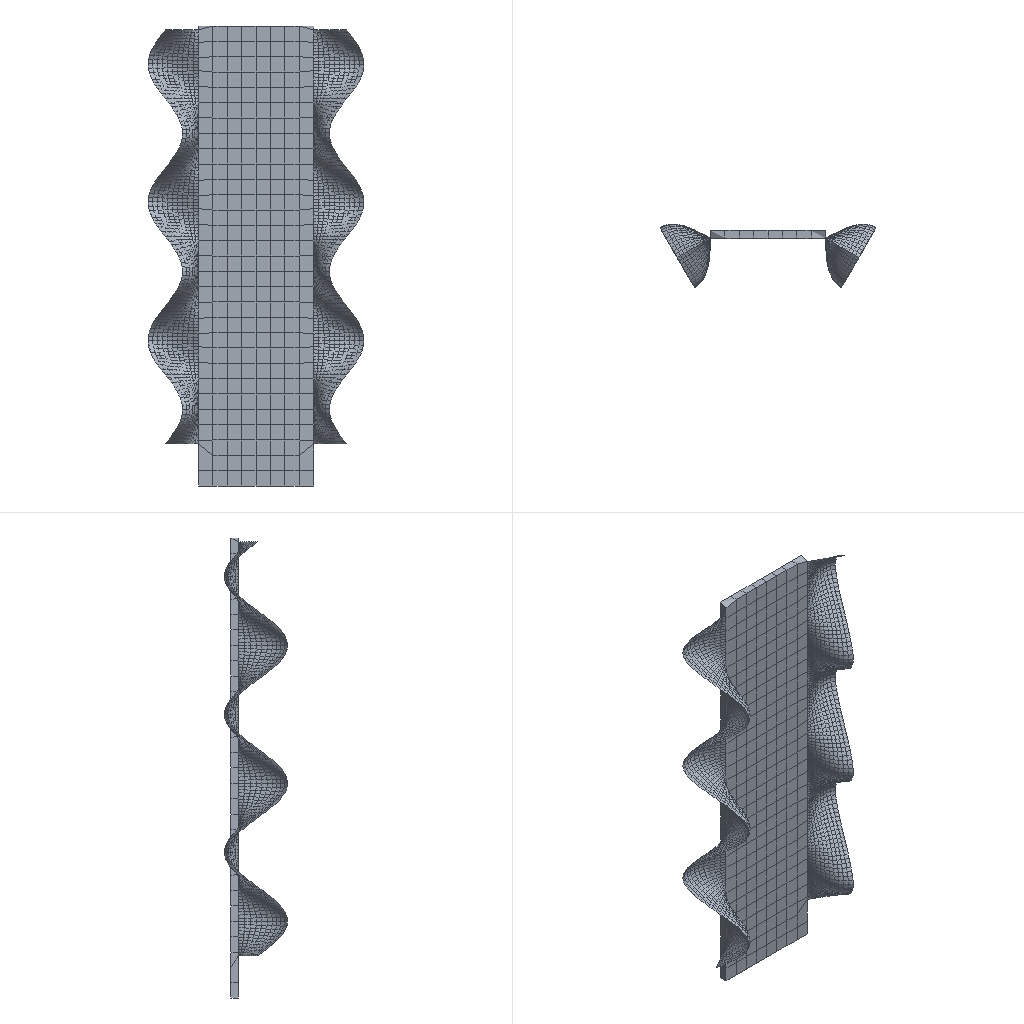Simulation study | abaqus
Set-up summary:
category,name,step,type,value,unit,region
solver,abaqus
solver,version,,,Abaqus/Explicit 2020
units,not stated in the deck,,not stated
analysis,deck,,transient,transient
load_step,Step-1,Step-1,transient
load_step,requested,,,1
mesh,nodes,,,4220
mesh,elements,,,3552
element_type,S4R,,shell,2640
element_type,R3D4,,rigid,672
element_type,C3D8R,,solid,240
load,load commands in deck,,count,3
bc,support commands in deck,,count,12
material,MATERIAL-1,,in results
check,setup vs results,,match,"per instance, exact: element labels, types and connectivity; labels of the nodes the elements use; coordinates not compared"
Abaqus input file, long lists of numbers shortened:
*Heading
** Job name: Job-2 Model name: Model-1
** Generated by: Abaqus/CAE 2020
*Preprint, echo=NO, model=NO, history=NO, contact=NO
**
** PARTS
**
*Part, name=body
*Node
      1,          12.,         -30.,           2.
      2,          12.,         -30.,           0.
** (556 more lines like these left out)
*Element, type=C3D8R
  1, 122, 130, 342, 181,   1,   2,  17,  62
  2, 181, 342, 343, 182,  62,  17,  18,  61
** (238 more lines like these left out)
*Nset, nset=Set-2, generate
   1,  558,    1
*Elset, elset=Set-2, generate
   1,  240,    1
*Nset, nset=Set-3, generate
   1,  558,    1
*Elset, elset=Set-3, generate
   1,  240,    1
** Section: Section-2
*Solid Section, elset=Set-3, material=Material-1
,
*End Part
**
*Part, name=merge
*Node
      1,           0.,           0.,          90.
      2,          10., 0.0001315,          90.
** (1461 more lines like these left out)
*Element, type=S4R
   1,    1,    8,  294,  177
   2,    8,    9,  295,  294
** (1318 more lines like these left out)
*Nset, nset=Set-3, generate
    1,  1463,     1
*Elset, elset=Set-3, generate
    1,  1320,     1
** Section: qiao
*Shell Section, elset=Set-3, material=Material-1
1., 5
*End Part
**
*Part, name=qi
*Node
      1,           0.,           0.,           0.
      2,           0.,           0., -0.8182
** (1461 more lines like these left out)
*Element, type=S4R
   1,    1,    2,  135,  134
   2,    2,    3,  136,  135
** (1318 more lines like these left out)
*Nset, nset=Set-1, generate
    1,  1463,     1
*Elset, elset=Set-1, generate
    1,  1320,     1
** Section: qiao
*Shell Section, elset=Set-1, material=Material-1
1., 5
*End Part
**
*Part, name=road
*Node
      1,         240.,        -27.5,           0.
      2,         235.,        -27.5,           0.
** (733 more lines like these left out)
*Element, type=R3D4
  1,   1,   2,  51,  50
  2,   2,   3,  52,  51
** (670 more lines like these left out)
*Node
    736,         120.,        -97.5,           0.
*Nset, nset=road-RefPt_, internal
736,
*Elset, elset=road, generate
   1,  672,    1
*End Part
**
**
** ASSEMBLY
**
*Assembly, name=Assembly
**
*Instance, name=qi-1, part=qi
  -49.16,    -14.706,    -1.
  -49.16,    -14.706,    -1.,   -49.16,    -14.706, -0.000292, 30.
*End Instance
**
*Instance, name=body-1, part=body
  -19.16,    -12.706, -0.000292
  -19.16,    -12.706, -0.000292, -18.583, -12.129, -0.5776,         120.
*End Instance
**
*Instance, name=merge-1, part=merge
  -19.16, -14.706,   -91.
  -19.16, -14.706,   -91.,   -19.16, -14.706, -92., 30.
*End Instance
**
*Instance, name=road-1, part=road
        27.5,        -27.5, 1.68388934882761e-15
        27.5,        -27.5, 1.68388934882761e-15, 28.077, -26.923, -0.5774,         120.
*End Instance
**
*Nset, nset=Set-1, instance=road-1, generate
   1,  735,    1
*Elset, elset=Set-1, instance=road-1, generate
   1,  672,    1
*Nset, nset=Set-6, instance=merge-1, generate
    1,  1463,     1
*Elset, elset=Set-6, instance=merge-1, generate
    1,  1320,     1
*Nset, nset=Set-7, instance=qi-1, generate
    1,  1463,     1
*Elset, elset=Set-7, instance=qi-1, generate
    1,  1320,     1
*Nset, nset=Set-8, instance=road-1
 736,
*Nset, nset=Set-9, instance=qi-1, generate
    1,  1463,     1
*Nset, nset=Set-9, instance=merge-1, generate
    1,  1463,     1
*Elset, elset=Set-9, instance=qi-1, generate
    1,  1320,     1
*Elset, elset=Set-9, instance=merge-1, generate
    1,  1320,     1
*Nset, nset=Set-11, instance=body-1
   2,   3,   5,   6,   9,  11,  14,  15,  17,  18,  19,  20,  21,  22,  23,  24
  25,  26,  27,  28,  29,  30,  31,  32,  33,  34,  35,  36,  37,  38,  39,  63
** (16 more lines like these left out)
*Elset, elset=Set-11, instance=body-1, generate
   1,  240,    1
*Nset, nset=m_Set-2, instance=qi-1, generate
   1,  133,    1
*Elset, elset=m_Set-2, instance=qi-1, generate
   1,  132,    1
*Nset, nset=m_Set-4, instance=merge-1
   1,   4,   5,   7, 135, 136, 137, 138, 139, 140, 141, 142, 143, 144, 145, 146
 147, 148, 149, 150, 151, 152, 153, 154, 155, 156, 157, 158, 159, 160, 161, 162
** (7 more lines like these left out)
*Elset, elset=m_Set-4, instance=merge-1
    1,   11,   21,   31,   41,   51,   61,   71,   81,   91,  101,  111,  121,  131,  141,  151
  161,  171,  181,  191,  201,  211,  221,  231,  241,  251,  261,  271,  281,  291,  301,  311
** (7 more lines like these left out)
*Nset, nset=s_Set-12, instance=body-1
   1,   4,  12,  16,  40,  41,  42,  43,  44,  45,  46,  47,  48,  49,  50,  51
  52,  53,  54,  55,  56,  57,  58,  59,  60,  61,  62, 143, 144, 175, 176
*Elset, elset=s_Set-12, instance=body-1
   1,   2,   3,   4,   5,   6,   7,   8,   9,  10,  11,  12,  13,  14,  15,  16
  17,  18,  19,  20,  21,  22,  23,  24, 214, 215, 216, 217, 225, 233
*Nset, nset=s_Set-13, instance=body-1
   7,   8,  10,  13,  86,  87,  88,  89,  90,  91,  92,  93,  94,  95,  96,  97
  98,  99, 100, 101, 102, 103, 104, 105, 106, 107, 108, 139, 140, 179, 180
*Elset, elset=s_Set-13, instance=body-1
 169, 170, 171, 172, 173, 174, 175, 176, 177, 178, 179, 180, 181, 182, 183, 184
 185, 186, 187, 188, 189, 190, 191, 192, 193, 194, 195, 224, 232, 240
*Elset, elset=_Surf-2_S5, internal, instance=body-1, generate
 217,  240,    1
*Surface, type=ELEMENT, name=Surf-2
_Surf-2_S5, S5
*Elset, elset=_Surf-3_E4, internal, instance=merge-1, generate
 1101,  1311,    10
*Surface, type=ELEMENT, name=Surf-3
_Surf-3_E4, E4
*Elset, elset=_Surf-4_E3, internal, instance=qi-1, generate
 1189,  1320,     1
*Surface, type=ELEMENT, name=Surf-4
_Surf-4_E3, E3
*Elset, elset=_Surf-5_S5, internal, instance=body-1, generate
 217,  240,    1
*Surface, type=ELEMENT, name=Surf-5
_Surf-5_S5, S5
*Elset, elset=_Surf-6_S5, internal, instance=body-1, generate
 217,  240,    1
*Elset, elset=_Surf-6_S4, internal, instance=body-1, generate
   1,  192,    1
*Surface, type=ELEMENT, name=Surf-6
_Surf-6_S5, S5
_Surf-6_S4, S4
*Surface, type=NODE, name=m_Set-2_CNS_, internal
m_Set-2, 1.
*Surface, type=NODE, name=s_Set-12_CNS_, internal
s_Set-12, 1.
*Surface, type=NODE, name=m_Set-4_CNS_, internal
m_Set-4, 1.
*Surface, type=NODE, name=s_Set-13_CNS_, internal
s_Set-13, 1.
*Rigid Body, ref node=road-1.road-RefPt_, elset=road-1.road
*Nset, nset="_T-Datum csys-2", internal
Set-6,
*Transform, nset="_T-Datum csys-2"
          0., 1.74937383367147e-08,           1.,           0.,           1., -1.74937383367147e-08
*Nset, nset="_T-Datum csys-3", internal
Set-7,
*Transform, nset="_T-Datum csys-3"
          1.,           0.,           0.,           0.,           1.,           0.
** Constraint: Constraint-1
*Tie, name=Constraint-1, adjust=yes
s_Set-12_CNS_, m_Set-2_CNS_
** Constraint: Constraint-2
*Tie, name=Constraint-2, adjust=yes
s_Set-13_CNS_, m_Set-4_CNS_
*End Assembly
*Amplitude, name=Amp-1
             0.,              0.,           0.001,              1.,           0.002,             -1.,           0.003,              1.
          0.004,             -1.,           0.005,              1.,           0.006,             -1.,           0.007,              1.
          0.008,             -1.,           0.009,              1.,            0.01,             -1.
*Amplitude, name=Amp-2
             0.,              0.,            0.01,              1.
**
** MATERIALS
**
*Material, name=Material-1
*Density
 2.6e-09,
*Elastic
1000., 0.4
**
** INTERACTION PROPERTIES
**
*Surface Interaction, name=IntProp-1
*Friction
 0.3,
*Surface Behavior, pressure-overclosure=HARD
** ----------------------------------------------------------------
**
** STEP: Step-1
**
*Step, name=Step-1, nlgeom=YES
*Dynamic, Explicit
, 0.01
*Bulk Viscosity
0.06, 1.2
**
** BOUNDARY CONDITIONS
**
** Name: BC-1 Type: 对称/反对称/完全固定
*Boundary
Set-8, ENCASTRE
** Name: BC-2 Type: 位移/转角
*Boundary, amplitude=Amp-1
Set-6, 4, 4, 0.5236
Set-6, 5, 5
Set-6, 6, 6
** Name: BC-3 Type: 位移/转角
*Boundary, amplitude=Amp-1
Set-7, 4, 4
Set-7, 5, 5
Set-7, 6, 6, -0.5236
** Name: BC-4 Type: 位移/转角
*Boundary
Set-11, 1, 1
Set-11, 2, 2
Set-11, 4, 4
Set-11, 5, 5
Set-11, 6, 6
**
** LOADS
**
** Name: Load-1   Type: Pressure
*Dsload
Surf-6, P, 0.6
**
** INTERACTIONS
**
** Interaction: Int-1
*Contact, op=NEW
*Contact Inclusions, ALL EXTERIOR
*Contact Property Assignment
 ,  , IntProp-1
**
** OUTPUT REQUESTS
**
*Restart, write, number interval=1, time marks=NO
**
** FIELD OUTPUT: F-Output-1
**
*Output, field, number interval=50
*Node Output
A, RF, U, V
*Element Output, directions=YES
E, EVF, LE, MISES, PE, PEEQ, PEEQVAVG, PEVAVG, S, SVAVG
*Contact Output
CSTRESS,
**
** HISTORY OUTPUT: H-Output-1
**
*Output, history, variable=PRESELECT
*End Step
Results summary:
result,step,Step-1,completed,increments=10691 time=0.01/0.01
result,analysis,,,transient
result,last_loadstep,,,1
result,primary field,,,"U, UR"
result,reaction total,,FX,185.555,model units
result,reaction total,,FY,1933.086,model units
result,reaction total,,FZ,-106.229,model units